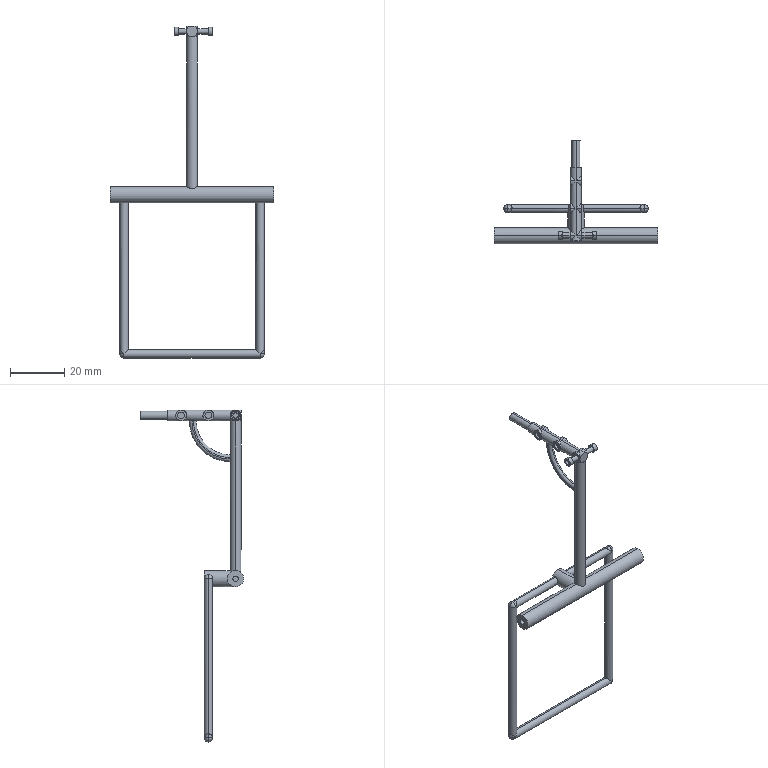Part | SolidWorks | features ICE 29, Fillet 5, Extrusion 1 | 2 solids | 133 faces | box 60 x 38 x 122 mm | volume 4628 mm3 | cylinder 78 | plane 35 | torus 12 | spline 8 | commonest cylinder face diameters 4 x31 3 x16 2 x14 2.5 x12 6 x5